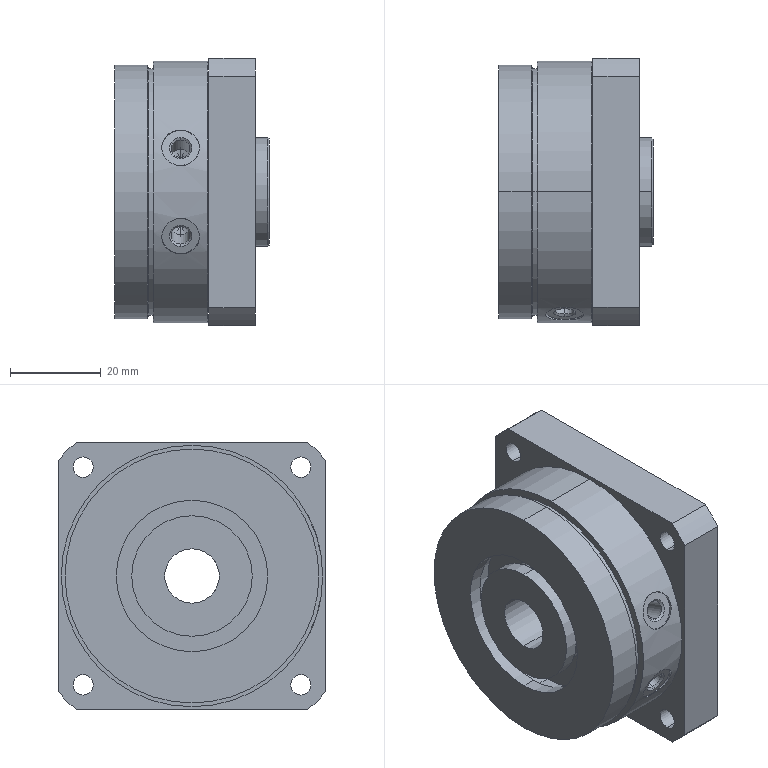Part | STEP file | PN_0054 | 1 solid | 78 faces | box 34 x 59 x 59 mm | volume 79656 mm3 | cylinder 44 | plane 20 | cone 12 | torus 2 | commonest cylinder face diameters 4.5 x8 24 x5 4.134 x4 8.3 x4 78 x4 12 x3